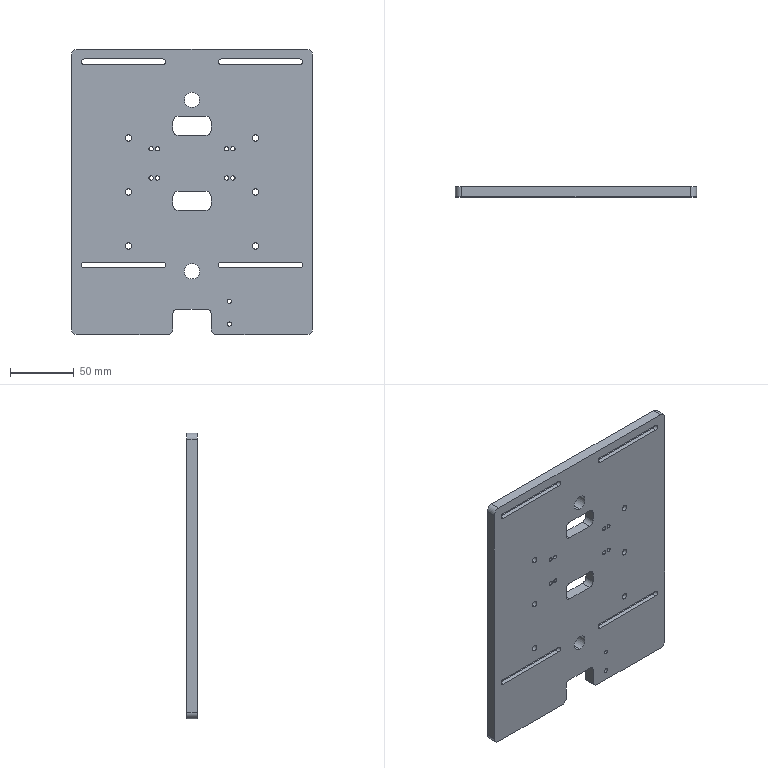Part | STEP file | 0-19-19 Mounting plate | 1 solid | 106 faces | box 190 x 8 x 225 mm | volume 312509 mm3 | cylinder 66 | plane 40 | commonest cylinder face diameters 3.3 x20 8 x16 5 x12 4.5 x8 10 x4 12 x4